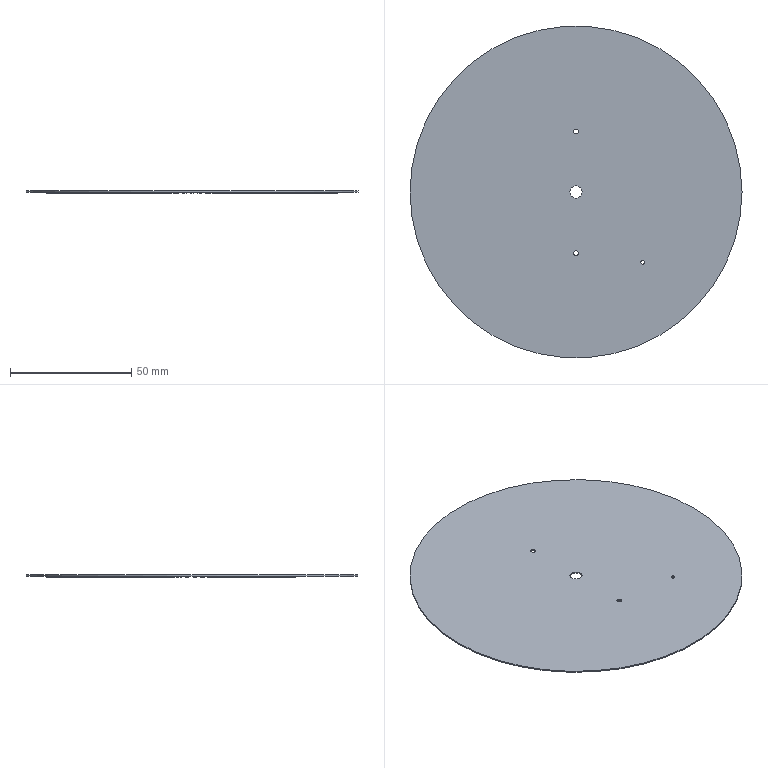Part | SolidWorks | features ICE 5, CirPattern 2, Cut 1, Extrusion 1 | 1 solid | 417 faces | box 137 x 137 x 1 mm | volume 7784 mm3 | plane 407 | cylinder 10 | commonest cylinder face diameters 2 x4 1.5 x2 5 x2 137 x2